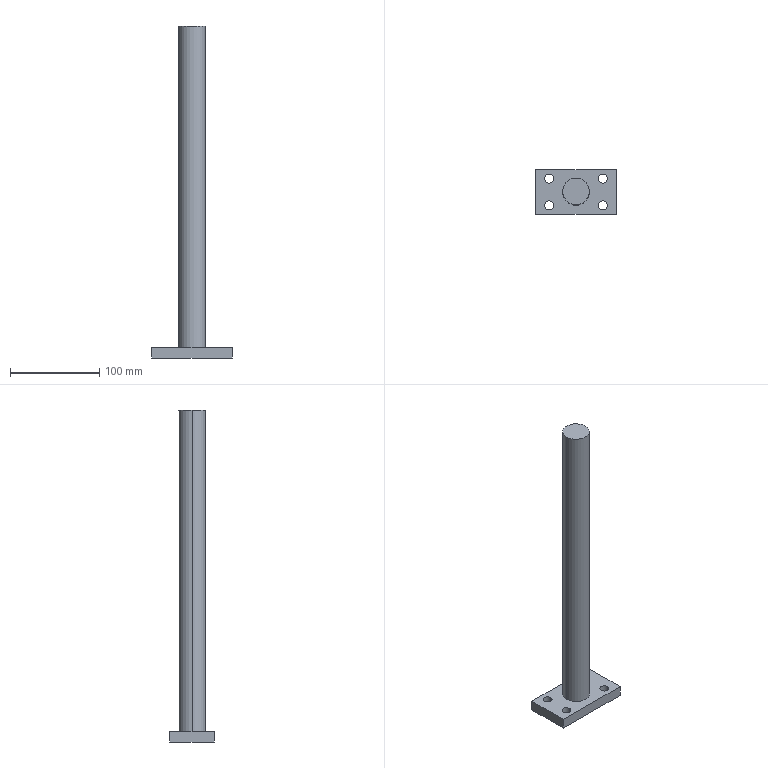Part | SolidWorks | features Extrusion 1, ICE 1 | 1 solid | 17 faces | box 90 x 50 x 372 mm | volume 304699 mm3 | cylinder 10 | plane 7 | commonest cylinder face diameters 10 x8 30 x2
STEP:
#1=CARTESIAN_POINT('',(15.,0.,372.));
#2=VERTEX_POINT('',#1);
#3=CARTESIAN_POINT('',(-15.,0.,372.));
#4=VERTEX_POINT('',#3);
#5=CARTESIAN_POINT('',(0.,0.,372.));
#6=DIRECTION('',(0.,0.,1.));
#7=DIRECTION('',(1.,0.,0.));
#8=AXIS2_PLACEMENT_3D('',#5,#6,#7);
#9=CIRCLE('',#8,15.);
#10=EDGE_CURVE('',#2,#4,#9,.T.);
#11=ORIENTED_EDGE('',*,*,#10,.F.);
#12=CARTESIAN_POINT('',(15.,0.,12.));
#13=VERTEX_POINT('',#12);
#14=CARTESIAN_POINT('',(15.,0.,372.));
#15=DIRECTION('',(0.,0.,-1.));
#16=VECTOR('',#15,1000.);
#17=LINE('',#14,#16);
#18=EDGE_CURVE('',#2,#13,#17,.T.);
#19=ORIENTED_EDGE('',*,*,#18,.T.);
#20=CARTESIAN_POINT('',(-15.,0.,12.));
#21=VERTEX_POINT('',#20);
#22=CARTESIAN_POINT('',(0.,0.,12.));
#23=DIRECTION('',(0.,0.,1.));
#24=DIRECTION('',(1.,0.,0.));
#25=AXIS2_PLACEMENT_3D('',#22,#23,#24);
#26=CIRCLE('',#25,15.);
#27=EDGE_CURVE('',#13,#21,#26,.T.);
#28=ORIENTED_EDGE('',*,*,#27,.T.);
#29=CARTESIAN_POINT('',(-15.,0.,372.));
#30=DIRECTION('',(0.,0.,-1.));
#31=VECTOR('',#30,1000.);
#32=LINE('',#29,#31);
#33=EDGE_CURVE('',#4,#21,#32,.T.);
#34=ORIENTED_EDGE('',*,*,#33,.F.);
#35=EDGE_LOOP('',(#11,#19,#28,#34));
#36=FACE_OUTER_BOUND('',#35,.T.);
#37=CARTESIAN_POINT('',(0.,0.,372.));
#38=DIRECTION('',(0.,0.,-1.));
#39=DIRECTION('',(-1.,0.,0.));
#40=AXIS2_PLACEMENT_3D('',#37,#38,#39);
#41=CYLINDRICAL_SURFACE('',#40,15.);
#42=ADVANCED_FACE('',(#36),#41,.T.);
#43=CARTESIAN_POINT('',(25.,15.,12.));
#44=VERTEX_POINT('',#43);
#45=CARTESIAN_POINT('',(35.,15.,12.));
#46=VERTEX_POINT('',#45);
#47=CARTESIAN_POINT('',(30.,15.,12.));
#48=DIRECTION('',(0.,0.,1.));
#49=DIRECTION('',(1.,0.,0.));
#50=AXIS2_PLACEMENT_3D('',#47,#48,#49);
#51=CIRCLE('',#50,5.);
#52=EDGE_CURVE('',#44,#46,#51,.T.);
#53=ORIENTED_EDGE('',*,*,#52,.T.);
#54=CARTESIAN_POINT('',(35.,15.,0.));
#55=VERTEX_POINT('',#54);
#56=CARTESIAN_POINT('',(35.,15.,12.));
#57=DIRECTION('',(0.,0.,-1.));
#58=VECTOR('',#57,1000.);
#59=LINE('',#56,#58);
#60=EDGE_CURVE('',#46,#55,#59,.T.);
#61=ORIENTED_EDGE('',*,*,#60,.T.);
#62=CARTESIAN_POINT('',(25.,15.,0.));
#63=VERTEX_POINT('',#62);
#64=CARTESIAN_POINT('',(30.,15.,0.));
#65=DIRECTION('',(0.,0.,1.));
#66=DIRECTION('',(1.,0.,0.));
#67=AXIS2_PLACEMENT_3D('',#64,#65,#66);
#68=CIRCLE('',#67,5.);
#69=EDGE_CURVE('',#63,#55,#68,.T.);
#70=ORIENTED_EDGE('',*,*,#69,.F.);
#71=CARTESIAN_POINT('',(25.,15.,12.));
#72=DIRECTION('',(0.,0.,-1.));
#73=VECTOR('',#72,1000.);
#74=LINE('',#71,#73);
#75=EDGE_CURVE('',#44,#63,#74,.T.);
#76=ORIENTED_EDGE('',*,*,#75,.F.);
#77=EDGE_LOOP('',(#53,#61,#70,#76));
#78=FACE_OUTER_BOUND('',#77,.T.);
#79=CARTESIAN_POINT('',(30.,15.,12.));
#80=DIRECTION('',(0.,0.,-1.));
#81=DIRECTION('',(-1.,0.,0.));
#82=AXIS2_PLACEMENT_3D('',#79,#80,#81);
#83=CYLINDRICAL_SURFACE('',#82,5.);
#84=ADVANCED_FACE('',(#78),#83,.F.);
#85=CARTESIAN_POINT('',(25.,-15.,12.));
#86=VERTEX_POINT('',#85);
#87=CARTESIAN_POINT('',(35.,-15.,12.));
#88=VERTEX_POINT('',#87);
#89=CARTESIAN_POINT('',(30.,-15.,12.));
#90=DIRECTION('',(0.,0.,1.));
#91=DIRECTION('',(1.,0.,0.));
#92=AXIS2_PLACEMENT_3D('',#89,#90,#91);
#93=CIRCLE('',#92,5.);
#94=EDGE_CURVE('',#86,#88,#93,.T.);
#95=ORIENTED_EDGE('',*,*,#94,.T.);
#96=CARTESIAN_POINT('',(35.,-15.,0.));
#97=VERTEX_POINT('',#96);
#98=CARTESIAN_POINT('',(35.,-15.,12.));
#99=DIRECTION('',(0.,0.,-1.));
#100=VECTOR('',#99,1000.);
#101=LINE('',#98,#100);
#102=EDGE_CURVE('',#88,#97,#101,.T.);
#103=ORIENTED_EDGE('',*,*,#102,.T.);
#104=CARTESIAN_POINT('',(25.,-15.,0.));
#105=VERTEX_POINT('',#104);
#106=CARTESIAN_POINT('',(30.,-15.,0.));
#107=DIRECTION('',(0.,0.,1.));
#108=DIRECTION('',(1.,0.,0.));
#109=AXIS2_PLACEMENT_3D('',#106,#107,#108);
#110=CIRCLE('',#109,5.);
#111=EDGE_CURVE('',#105,#97,#110,.T.);
#112=ORIENTED_EDGE('',*,*,#111,.F.);
#113=CARTESIAN_POINT('',(25.,-15.,12.));
#114=DIRECTION('',(0.,0.,-1.));
#115=VECTOR('',#114,1000.);
#116=LINE('',#113,#115);
#117=EDGE_CURVE('',#86,#105,#116,.T.);
#118=ORIENTED_EDGE('',*,*,#117,.F.);
#119=EDGE_LOOP('',(#95,#103,#112,#118));
#120=FACE_OUTER_BOUND('',#119,.T.);
#121=CARTESIAN_POINT('',(30.,-15.,12.));
#122=DIRECTION('',(0.,0.,-1.));
#123=DIRECTION('',(-1.,0.,0.));
#124=AXIS2_PLACEMENT_3D('',#121,#122,#123);
#125=CYLINDRICAL_SURFACE('',#124,5.);
#126=ADVANCED_FACE('',(#120),#125,.F.);
#127=CARTESIAN_POINT('',(-35.,-15.,12.));
#128=VERTEX_POINT('',#127);
#129=CARTESIAN_POINT('',(-25.,-15.,12.));
#130=VERTEX_POINT('',#129);
#131=CARTESIAN_POINT('',(-30.,-15.,12.));
#132=DIRECTION('',(0.,0.,1.));
#133=DIRECTION('',(1.,0.,0.));
#134=AXIS2_PLACEMENT_3D('',#131,#132,#133);
#135=CIRCLE('',#134,5.);
#136=EDGE_CURVE('',#128,#130,#135,.T.);
#137=ORIENTED_EDGE('',*,*,#136,.T.);
#138=CARTESIAN_POINT('',(-25.,-15.,0.));
#139=VERTEX_POINT('',#138);
#140=CARTESIAN_POINT('',(-25.,-15.,12.));
#141=DIRECTION('',(0.,0.,-1.));
#142=VECTOR('',#141,1000.);
#143=LINE('',#140,#142);
#144=EDGE_CURVE('',#130,#139,#143,.T.);
#145=ORIENTED_EDGE('',*,*,#144,.T.);
#146=CARTESIAN_POINT('',(-35.,-15.,0.));
#147=VERTEX_POINT('',#146);
#148=CARTESIAN_POINT('',(-30.,-15.,0.));
#149=DIRECTION('',(0.,0.,1.));
#150=DIRECTION('',(1.,0.,0.));
#151=AXIS2_PLACEMENT_3D('',#148,#149,#150);
#152=CIRCLE('',#151,5.);
#153=EDGE_CURVE('',#147,#139,#152,.T.);
#154=ORIENTED_EDGE('',*,*,#153,.F.);
#155=CARTESIAN_POINT('',(-35.,-15.,12.));
#156=DIRECTION('',(0.,0.,-1.));
#157=VECTOR('',#156,1000.);
#158=LINE('',#155,#157);
#159=EDGE_CURVE('',#128,#147,#158,.T.);
#160=ORIENTED_EDGE('',*,*,#159,.F.);
#161=EDGE_LOOP('',(#137,#145,#154,#160));
#162=FACE_OUTER_BOUND('',#161,.T.);
#163=CARTESIAN_POINT('',(-30.,-15.,12.));
#164=DIRECTION('',(0.,0.,-1.));
#165=DIRECTION('',(-1.,0.,0.));
#166=AXIS2_PLACEMENT_3D('',#163,#164,#165);
#167=CYLINDRICAL_SURFACE('',#166,5.);
#168=ADVANCED_FACE('',(#162),#167,.F.);
#169=CARTESIAN_POINT('',(-35.,15.,12.));
#170=VERTEX_POINT('',#169);
#171=CARTESIAN_POINT('',(-25.,15.,12.));
#172=VERTEX_POINT('',#171);
#173=CARTESIAN_POINT('',(-30.,15.,12.));
#174=DIRECTION('',(0.,0.,1.));
#175=DIRECTION('',(1.,0.,0.));
#176=AXIS2_PLACEMENT_3D('',#173,#174,#175);
#177=CIRCLE('',#176,5.);
#178=EDGE_CURVE('',#170,#172,#177,.T.);
#179=ORIENTED_EDGE('',*,*,#178,.T.);
#180=CARTESIAN_POINT('',(-25.,15.,0.));
#181=VERTEX_POINT('',#180);
#182=CARTESIAN_POINT('',(-25.,15.,12.));
#183=DIRECTION('',(0.,0.,-1.));
#184=VECTOR('',#183,1000.);
#185=LINE('',#182,#184);
#186=EDGE_CURVE('',#172,#181,#185,.T.);
#187=ORIENTED_EDGE('',*,*,#186,.T.);
#188=CARTESIAN_POINT('',(-35.,15.,0.));
#189=VERTEX_POINT('',#188);
#190=CARTESIAN_POINT('',(-30.,15.,0.));
#191=DIRECTION('',(0.,0.,1.));
#192=DIRECTION('',(1.,0.,0.));
#193=AXIS2_PLACEMENT_3D('',#190,#191,#192);
#194=CIRCLE('',#193,5.);
#195=EDGE_CURVE('',#189,#181,#194,.T.);
#196=ORIENTED_EDGE('',*,*,#195,.F.);
#197=CARTESIAN_POINT('',(-35.,15.,12.));
#198=DIRECTION('',(0.,0.,-1.));
#199=VECTOR('',#198,1000.);
#200=LINE('',#197,#199);
#201=EDGE_CURVE('',#170,#189,#200,.T.);
#202=ORIENTED_EDGE('',*,*,#201,.F.);
#203=EDGE_LOOP('',(#179,#187,#196,#202));
#204=FACE_OUTER_BOUND('',#203,.T.);
#205=CARTESIAN_POINT('',(-30.,15.,12.));
#206=DIRECTION('',(0.,0.,-1.));
#207=DIRECTION('',(-1.,0.,0.));
#208=AXIS2_PLACEMENT_3D('',#205,#206,#207);
#209=CYLINDRICAL_SURFACE('',#208,5.);
#210=ADVANCED_FACE('',(#204),#209,.F.);
#211=CARTESIAN_POINT('',(0.,0.,12.));
#212=DIRECTION('',(0.,0.,1.));
#213=DIRECTION('',(1.,0.,0.));
#214=AXIS2_PLACEMENT_3D('',#211,#212,#213);
#215=CIRCLE('',#214,15.);
#216=EDGE_CURVE('',#21,#13,#215,.T.);
#217=ORIENTED_EDGE('',*,*,#216,.F.);
#218=ORIENTED_EDGE('',*,*,#27,.F.);
#219=EDGE_LOOP('',(#217,#218));
#220=FACE_BOUND('',#219,.T.);
#221=ORIENTED_EDGE('',*,*,#94,.F.);
#222=CARTESIAN_POINT('',(30.,-15.,12.));
#223=DIRECTION('',(0.,0.,1.));
#224=DIRECTION('',(1.,0.,0.));
#225=AXIS2_PLACEMENT_3D('',#222,#223,#224);
#226=CIRCLE('',#225,5.);
#227=EDGE_CURVE('',#88,#86,#226,.T.);
#228=ORIENTED_EDGE('',*,*,#227,.F.);
#229=EDGE_LOOP('',(#221,#228));
#230=FACE_BOUND('',#229,.T.);
#231=ORIENTED_EDGE('',*,*,#178,.F.);
#232=CARTESIAN_POINT('',(-30.,15.,12.));
#233=DIRECTION('',(0.,0.,1.));
#234=DIRECTION('',(1.,0.,0.));
#235=AXIS2_PLACEMENT_3D('',#232,#233,#234);
#236=CIRCLE('',#235,5.);
#237=EDGE_CURVE('',#172,#170,#236,.T.);
#238=ORIENTED_EDGE('',*,*,#237,.F.);
#239=EDGE_LOOP('',(#231,#238));
#240=FACE_BOUND('',#239,.T.);
#241=CARTESIAN_POINT('',(45.,-25.,12.));
#242=VERTEX_POINT('',#241);
#243=CARTESIAN_POINT('',(45.,25.,12.));
#244=VERTEX_POINT('',#243);
#245=CARTESIAN_POINT('',(45.,25.,12.));
#246=DIRECTION('',(0.,1.,0.));
#247=VECTOR('',#246,1000.);
#248=LINE('',#245,#247);
#249=EDGE_CURVE('',#242,#244,#248,.T.);
#250=ORIENTED_EDGE('',*,*,#249,.T.);
#251=CARTESIAN_POINT('',(-45.,25.,12.));
#252=VERTEX_POINT('',#251);
#253=CARTESIAN_POINT('',(-45.,25.,12.));
#254=DIRECTION('',(-1.,0.,0.));
#255=VECTOR('',#254,1000.);
#256=LINE('',#253,#255);
#257=EDGE_CURVE('',#244,#252,#256,.T.);
#258=ORIENTED_EDGE('',*,*,#257,.T.);
#259=CARTESIAN_POINT('',(-45.,-25.,12.));
#260=VERTEX_POINT('',#259);
#261=CARTESIAN_POINT('',(-45.,25.,12.));
#262=DIRECTION('',(0.,-1.,0.));
#263=VECTOR('',#262,1000.);
#264=LINE('',#261,#263);
#265=EDGE_CURVE('',#252,#260,#264,.T.);
#266=ORIENTED_EDGE('',*,*,#265,.T.);
#267=CARTESIAN_POINT('',(-45.,-25.,12.));
#268=DIRECTION('',(1.,0.,0.));
#269=VECTOR('',#268,1000.);
#270=LINE('',#267,#269);
#271=EDGE_CURVE('',#260,#242,#270,.T.);
#272=ORIENTED_EDGE('',*,*,#271,.T.);
#273=EDGE_LOOP('',(#250,#258,#266,#272));
#274=FACE_OUTER_BOUND('',#273,.T.);
#275=ORIENTED_EDGE('',*,*,#136,.F.);
#276=CARTESIAN_POINT('',(-30.,-15.,12.));
#277=DIRECTION('',(0.,0.,1.));
#278=DIRECTION('',(1.,0.,0.));
#279=AXIS2_PLACEMENT_3D('',#276,#277,#278);
#280=CIRCLE('',#279,5.);
#281=EDGE_CURVE('',#130,#128,#280,.T.);
#282=ORIENTED_EDGE('',*,*,#281,.F.);
#283=EDGE_LOOP('',(#275,#282));
#284=FACE_BOUND('',#283,.T.);
#285=ORIENTED_EDGE('',*,*,#52,.F.);
#286=CARTESIAN_POINT('',(30.,15.,12.));
#287=DIRECTION('',(0.,0.,1.));
#288=DIRECTION('',(1.,0.,0.));
#289=AXIS2_PLACEMENT_3D('',#286,#287,#288);
#290=CIRCLE('',#289,5.);
#291=EDGE_CURVE('',#46,#44,#290,.T.);
#292=ORIENTED_EDGE('',*,*,#291,.F.);
#293=EDGE_LOOP('',(#285,#292));
#294=FACE_BOUND('',#293,.T.);
#295=CARTESIAN_POINT('',(0.,0.,12.));
#296=DIRECTION('',(0.,0.,1.));
#297=DIRECTION('',(1.,0.,0.));
#298=AXIS2_PLACEMENT_3D('',#295,#296,#297);
#299=PLANE('',#298);
#300=ADVANCED_FACE('',(#220,#230,#240,#274,#284,#294),#299,.T.);
#301=CARTESIAN_POINT('',(45.,-25.,0.));
#302=VERTEX_POINT('',#301);
#303=CARTESIAN_POINT('',(45.,25.,0.));
#304=VERTEX_POINT('',#303);
#305=CARTESIAN_POINT('',(45.,25.,0.));
#306=DIRECTION('',(0.,1.,0.));
#307=VECTOR('',#306,1000.);
#308=LINE('',#305,#307);
#309=EDGE_CURVE('',#302,#304,#308,.T.);
#310=ORIENTED_EDGE('',*,*,#309,.F.);
#311=CARTESIAN_POINT('',(-45.,-25.,0.));
#312=VERTEX_POINT('',#311);
#313=CARTESIAN_POINT('',(-45.,-25.,0.));
#314=DIRECTION('',(1.,0.,0.));
#315=VECTOR('',#314,1000.);
#316=LINE('',#313,#315);
#317=EDGE_CURVE('',#312,#302,#316,.T.);
#318=ORIENTED_EDGE('',*,*,#317,.F.);
#319=CARTESIAN_POINT('',(-45.,25.,0.));
#320=VERTEX_POINT('',#319);
#321=CARTESIAN_POINT('',(-45.,25.,0.));
#322=DIRECTION('',(0.,-1.,0.));
#323=VECTOR('',#322,1000.);
#324=LINE('',#321,#323);
#325=EDGE_CURVE('',#320,#312,#324,.T.);
#326=ORIENTED_EDGE('',*,*,#325,.F.);
#327=CARTESIAN_POINT('',(-45.,25.,0.));
#328=DIRECTION('',(-1.,0.,0.));
#329=VECTOR('',#328,1000.);
#330=LINE('',#327,#329);
#331=EDGE_CURVE('',#304,#320,#330,.T.);
#332=ORIENTED_EDGE('',*,*,#331,.F.);
#333=EDGE_LOOP('',(#310,#318,#326,#332));
#334=FACE_OUTER_BOUND('',#333,.T.);
#335=ORIENTED_EDGE('',*,*,#195,.T.);
#336=CARTESIAN_POINT('',(-30.,15.,0.));
#337=DIRECTION('',(0.,0.,1.));
#338=DIRECTION('',(1.,0.,0.));
#339=AXIS2_PLACEMENT_3D('',#336,#337,#338);
#340=CIRCLE('',#339,5.);
#341=EDGE_CURVE('',#181,#189,#340,.T.);
#342=ORIENTED_EDGE('',*,*,#341,.T.);
#343=EDGE_LOOP('',(#335,#342));
#344=FACE_BOUND('',#343,.T.);
#345=ORIENTED_EDGE('',*,*,#153,.T.);
#346=CARTESIAN_POINT('',(-30.,-15.,0.));
#347=DIRECTION('',(0.,0.,1.));
#348=DIRECTION('',(1.,0.,0.));
#349=AXIS2_PLACEMENT_3D('',#346,#347,#348);
#350=CIRCLE('',#349,5.);
#351=EDGE_CURVE('',#139,#147,#350,.T.);
#352=ORIENTED_EDGE('',*,*,#351,.T.);
#353=EDGE_LOOP('',(#345,#352));
#354=FACE_BOUND('',#353,.T.);
#355=ORIENTED_EDGE('',*,*,#111,.T.);
#356=CARTESIAN_POINT('',(30.,-15.,0.));
#357=DIRECTION('',(0.,0.,1.));
#358=DIRECTION('',(1.,0.,0.));
#359=AXIS2_PLACEMENT_3D('',#356,#357,#358);
#360=CIRCLE('',#359,5.);
#361=EDGE_CURVE('',#97,#105,#360,.T.);
#362=ORIENTED_EDGE('',*,*,#361,.T.);
#363=EDGE_LOOP('',(#355,#362));
#364=FACE_BOUND('',#363,.T.);
#365=ORIENTED_EDGE('',*,*,#69,.T.);
#366=CARTESIAN_POINT('',(30.,15.,0.));
#367=DIRECTION('',(0.,0.,1.));
#368=DIRECTION('',(1.,0.,0.));
#369=AXIS2_PLACEMENT_3D('',#366,#367,#368);
#370=CIRCLE('',#369,5.);
#371=EDGE_CURVE('',#55,#63,#370,.T.);
#372=ORIENTED_EDGE('',*,*,#371,.T.);
#373=EDGE_LOOP('',(#365,#372));
#374=FACE_BOUND('',#373,.T.);
#375=CARTESIAN_POINT('',(0.,0.,0.));
#376=DIRECTION('',(0.,0.,1.));
#377=DIRECTION('',(1.,0.,0.));
#378=AXIS2_PLACEMENT_3D('',#375,#376,#377);
#379=PLANE('',#378);
#380=ADVANCED_FACE('',(#334,#344,#354,#364,#374),#379,.F.);
#381=ORIENTED_EDGE('',*,*,#309,.T.);
#382=CARTESIAN_POINT('',(45.,25.,12.));
#383=DIRECTION('',(0.,0.,-1.));
#384=VECTOR('',#383,1000.);
#385=LINE('',#382,#384);
#386=EDGE_CURVE('',#244,#304,#385,.T.);
#387=ORIENTED_EDGE('',*,*,#386,.F.);
#388=ORIENTED_EDGE('',*,*,#249,.F.);
#389=CARTESIAN_POINT('',(45.,-25.,12.));
#390=DIRECTION('',(0.,0.,-1.));
#391=VECTOR('',#390,1000.);
#392=LINE('',#389,#391);
#393=EDGE_CURVE('',#242,#302,#392,.T.);
#394=ORIENTED_EDGE('',*,*,#393,.T.);
#395=EDGE_LOOP('',(#381,#387,#388,#394));
#396=FACE_OUTER_BOUND('',#395,.T.);
#397=CARTESIAN_POINT('',(45.,25.,12.));
#398=DIRECTION('',(-1.,0.,0.));
#399=DIRECTION('',(0.,-1.,0.));
#400=AXIS2_PLACEMENT_3D('',#397,#398,#399);
#401=PLANE('',#400);
#402=ADVANCED_FACE('',(#396),#401,.F.);
#403=ORIENTED_EDGE('',*,*,#331,.T.);
#404=CARTESIAN_POINT('',(-45.,25.,12.));
#405=DIRECTION('',(0.,0.,-1.));
#406=VECTOR('',#405,1000.);
#407=LINE('',#404,#406);
#408=EDGE_CURVE('',#252,#320,#407,.T.);
#409=ORIENTED_EDGE('',*,*,#408,.F.);
#410=ORIENTED_EDGE('',*,*,#257,.F.);
#411=ORIENTED_EDGE('',*,*,#386,.T.);
#412=EDGE_LOOP('',(#403,#409,#410,#411));
#413=FACE_OUTER_BOUND('',#412,.T.);
#414=CARTESIAN_POINT('',(-45.,25.,12.));
#415=DIRECTION('',(0.,-1.,0.));
#416=DIRECTION('',(0.,0.,-1.));
#417=AXIS2_PLACEMENT_3D('',#414,#415,#416);
#418=PLANE('',#417);
#419=ADVANCED_FACE('',(#413),#418,.F.);
#420=ORIENTED_EDGE('',*,*,#325,.T.);
#421=CARTESIAN_POINT('',(-45.,-25.,12.));
#422=DIRECTION('',(0.,0.,-1.));
#423=VECTOR('',#422,1000.);
#424=LINE('',#421,#423);
#425=EDGE_CURVE('',#260,#312,#424,.T.);
#426=ORIENTED_EDGE('',*,*,#425,.F.);
#427=ORIENTED_EDGE('',*,*,#265,.F.);
#428=ORIENTED_EDGE('',*,*,#408,.T.);
#429=EDGE_LOOP('',(#420,#426,#427,#428));
#430=FACE_OUTER_BOUND('',#429,.T.);
#431=CARTESIAN_POINT('',(-45.,25.,12.));
#432=DIRECTION('',(1.,0.,0.));
#433=DIRECTION('',(0.,0.,-1.));
#434=AXIS2_PLACEMENT_3D('',#431,#432,#433);
#435=PLANE('',#434);
#436=ADVANCED_FACE('',(#430),#435,.F.);
#437=ORIENTED_EDGE('',*,*,#317,.T.);
#438=ORIENTED_EDGE('',*,*,#393,.F.);
#439=ORIENTED_EDGE('',*,*,#271,.F.);
#440=ORIENTED_EDGE('',*,*,#425,.T.);
#441=EDGE_LOOP('',(#437,#438,#439,#440));
#442=FACE_OUTER_BOUND('',#441,.T.);
#443=CARTESIAN_POINT('',(-45.,-25.,12.));
#444=DIRECTION('',(0.,1.,0.));
#445=DIRECTION('',(0.,0.,1.));
#446=AXIS2_PLACEMENT_3D('',#443,#444,#445);
#447=PLANE('',#446);
#448=ADVANCED_FACE('',(#442),#447,.F.);
#449=ORIENTED_EDGE('',*,*,#186,.F.);
#450=ORIENTED_EDGE('',*,*,#237,.T.);
#451=ORIENTED_EDGE('',*,*,#201,.T.);
#452=ORIENTED_EDGE('',*,*,#341,.F.);
#453=EDGE_LOOP('',(#449,#450,#451,#452));
#454=FACE_OUTER_BOUND('',#453,.T.);
#455=CARTESIAN_POINT('',(-30.,15.,12.));
#456=DIRECTION('',(0.,0.,-1.));
#457=DIRECTION('',(-1.,0.,0.));
#458=AXIS2_PLACEMENT_3D('',#455,#456,#457);
#459=CYLINDRICAL_SURFACE('',#458,5.);
#460=ADVANCED_FACE('',(#454),#459,.F.);
#461=ORIENTED_EDGE('',*,*,#144,.F.);
#462=ORIENTED_EDGE('',*,*,#281,.T.);
#463=ORIENTED_EDGE('',*,*,#159,.T.);
#464=ORIENTED_EDGE('',*,*,#351,.F.);
#465=EDGE_LOOP('',(#461,#462,#463,#464));
#466=FACE_OUTER_BOUND('',#465,.T.);
#467=CARTESIAN_POINT('',(-30.,-15.,12.));
#468=DIRECTION('',(0.,0.,-1.));
#469=DIRECTION('',(-1.,0.,0.));
#470=AXIS2_PLACEMENT_3D('',#467,#468,#469);
#471=CYLINDRICAL_SURFACE('',#470,5.);
#472=ADVANCED_FACE('',(#466),#471,.F.);
#473=ORIENTED_EDGE('',*,*,#102,.F.);
#474=ORIENTED_EDGE('',*,*,#227,.T.);
#475=ORIENTED_EDGE('',*,*,#117,.T.);
#476=ORIENTED_EDGE('',*,*,#361,.F.);
#477=EDGE_LOOP('',(#473,#474,#475,#476));
#478=FACE_OUTER_BOUND('',#477,.T.);
#479=CARTESIAN_POINT('',(30.,-15.,12.));
#480=DIRECTION('',(0.,0.,-1.));
#481=DIRECTION('',(-1.,0.,0.));
#482=AXIS2_PLACEMENT_3D('',#479,#480,#481);
#483=CYLINDRICAL_SURFACE('',#482,5.);
#484=ADVANCED_FACE('',(#478),#483,.F.);
#485=ORIENTED_EDGE('',*,*,#60,.F.);
#486=ORIENTED_EDGE('',*,*,#291,.T.);
#487=ORIENTED_EDGE('',*,*,#75,.T.);
#488=ORIENTED_EDGE('',*,*,#371,.F.);
#489=EDGE_LOOP('',(#485,#486,#487,#488));
#490=FACE_OUTER_BOUND('',#489,.T.);
#491=CARTESIAN_POINT('',(30.,15.,12.));
#492=DIRECTION('',(0.,0.,-1.));
#493=DIRECTION('',(-1.,0.,0.));
#494=AXIS2_PLACEMENT_3D('',#491,#492,#493);
#495=CYLINDRICAL_SURFACE('',#494,5.);
#496=ADVANCED_FACE('',(#490),#495,.F.);
#497=ORIENTED_EDGE('',*,*,#18,.F.);
#498=CARTESIAN_POINT('',(0.,0.,372.));
#499=DIRECTION('',(0.,0.,1.));
#500=DIRECTION('',(1.,0.,0.));
#501=AXIS2_PLACEMENT_3D('',#498,#499,#500);
#502=CIRCLE('',#501,15.);
#503=EDGE_CURVE('',#4,#2,#502,.T.);
#504=ORIENTED_EDGE('',*,*,#503,.F.);
#505=ORIENTED_EDGE('',*,*,#33,.T.);
#506=ORIENTED_EDGE('',*,*,#216,.T.);
#507=EDGE_LOOP('',(#497,#504,#505,#506));
#508=FACE_OUTER_BOUND('',#507,.T.);
#509=CARTESIAN_POINT('',(0.,0.,372.));
#510=DIRECTION('',(0.,0.,-1.));
#511=DIRECTION('',(-1.,0.,0.));
#512=AXIS2_PLACEMENT_3D('',#509,#510,#511);
#513=CYLINDRICAL_SURFACE('',#512,15.);
#514=ADVANCED_FACE('',(#508),#513,.T.);
#515=ORIENTED_EDGE('',*,*,#503,.T.);
#516=ORIENTED_EDGE('',*,*,#10,.T.);
#517=EDGE_LOOP('',(#515,#516));
#518=FACE_OUTER_BOUND('',#517,.T.);
#519=CARTESIAN_POINT('',(0.,0.,372.));
#520=DIRECTION('',(0.,0.,1.));
#521=DIRECTION('',(1.,0.,0.));
#522=AXIS2_PLACEMENT_3D('',#519,#520,#521);
#523=PLANE('',#522);
#524=ADVANCED_FACE('',(#518),#523,.T.);
#525=CLOSED_SHELL('',(#42,#84,#126,#168,#210,#300,#380,#402,#419,#436,#448,#460,#472,#484,#496,#514,#524));
#526=MANIFOLD_SOLID_BREP('',#525);
#527=CARTESIAN_POINT('',(0.,0.,0.));
#528=DIRECTION('',(0.,0.,1.));
#529=DIRECTION('',(1.,0.,0.));
#530=AXIS2_PLACEMENT_3D('',#527,#528,#529);
#531=(LENGTH_UNIT()NAMED_UNIT(*)SI_UNIT(.MILLI.,.METRE.));
#532=UNCERTAINTY_MEASURE_WITH_UNIT(LENGTH_MEASURE(0.00001),#531,'','');
#533=(NAMED_UNIT(*)PLANE_ANGLE_UNIT()SI_UNIT($,.RADIAN.));
#534=(NAMED_UNIT(*)SI_UNIT($,.STERADIAN.)SOLID_ANGLE_UNIT());
#535=(GEOMETRIC_REPRESENTATION_CONTEXT(3)GLOBAL_UNCERTAINTY_ASSIGNED_CONTEXT((#532))GLOBAL_UNIT_ASSIGNED_CONTEXT((#531,#533,#534))REPRESENTATION_CONTEXT('',''));
#536=ADVANCED_BREP_SHAPE_REPRESENTATION('',(#526,#530),#535);